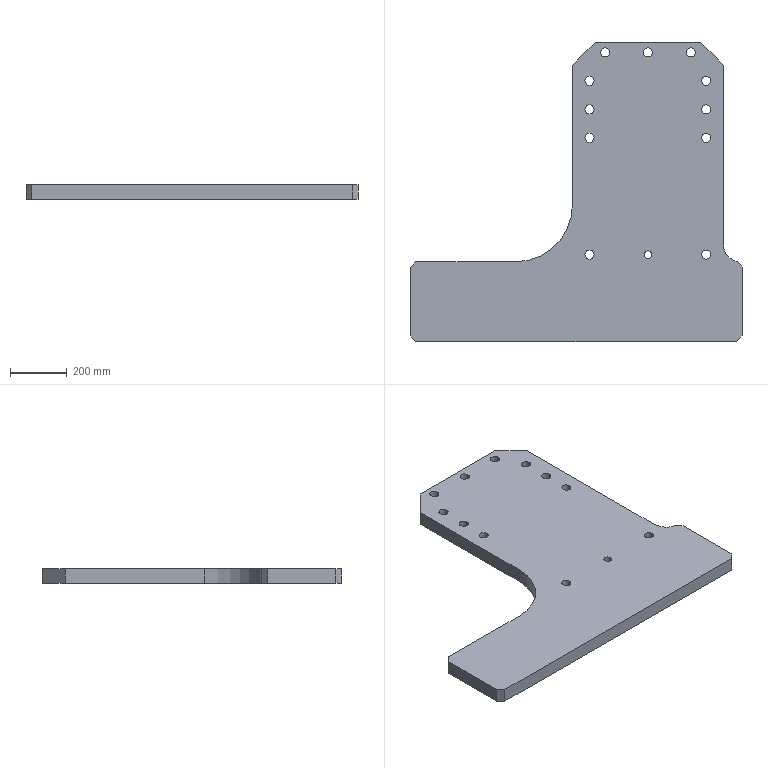Part | SolidWorks | features Chamfer 3, ICE 2, 3DProfileFeature 1, Extrusion 1, HoleWzd 1 | 1 solid | 53 faces | box 1165 x 1050 x 50 mm | volume 36177793 mm3 | cylinder 30 | plane 17 | cone 6 | commonest cylinder face diameters 32 x22 75 x4 26.5 x2 120 x1 400 x1